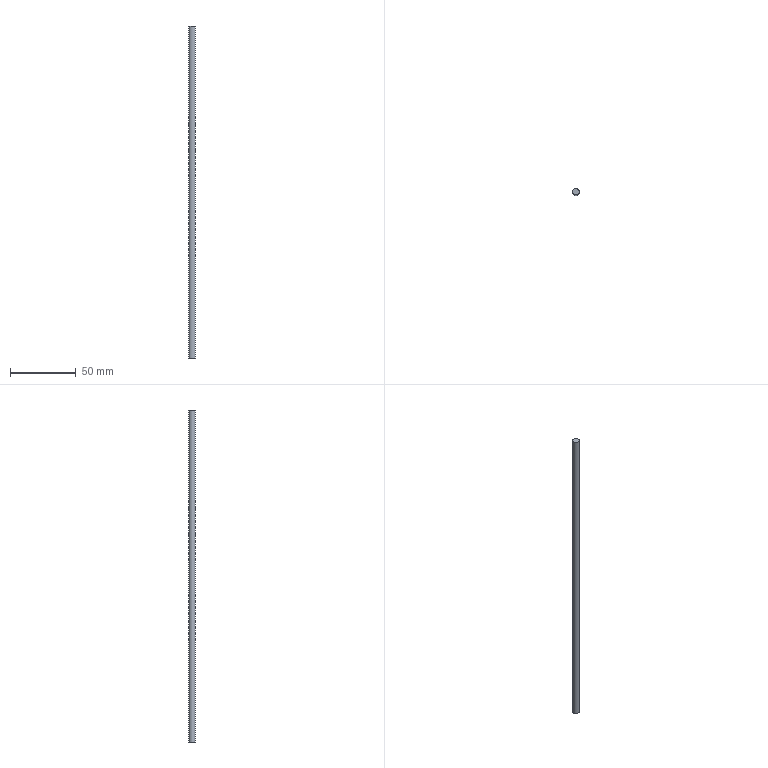Part | STEP file | gslz 2016.10.28-13_id302_x_t | 1 solid | 3 faces | box 5 x 5 x 252 mm | volume 4948 mm3 | plane 2 | cylinder 1 | commonest cylinder face diameters 5 x1
STEP:
#1=CARTESIAN_POINT('',(0.,0.,0.));
#2=DIRECTION('',(0.,0.,1.));
#3=DIRECTION('',(1.,0.,0.));
#4=AXIS2_PLACEMENT_3D('',#1,#2,#3);
#5=CARTESIAN_POINT('',(-229.514,212.012,73.));
#6=VERTEX_POINT('',#5);
#7=CARTESIAN_POINT('',(-234.496,212.311,73.));
#8=VERTEX_POINT('',#7);
#9=CARTESIAN_POINT('',(-232.014,212.012,73.));
#10=DIRECTION('',(0.,0.,-1.));
#11=DIRECTION('',(1.,0.,0.));
#12=AXIS2_PLACEMENT_3D('',#9,#10,#11);
#13=CIRCLE('',#12,2.5);
#14=CARTESIAN_POINT('',(-232.014,212.012,21.));
#15=DIRECTION('',(0.,0.,-1.));
#16=DIRECTION('',(0.,1.,0.));
#17=AXIS2_PLACEMENT_3D('',#14,#15,#16);
#18=CYLINDRICAL_SURFACE('',#17,2.5);
#19=CARTESIAN_POINT('',(7.854,-52.));
#20=DIRECTION('',(1.,0.));
#21=VECTOR('',#20,1.);
#22=LINE('',#19,#21);
#23=(GEOMETRIC_REPRESENTATION_CONTEXT(2)PARAMETRIC_REPRESENTATION_CONTEXT()REPRESENTATION_CONTEXT('',''));
#24=DEFINITIONAL_REPRESENTATION('',(#22),#23);
#25=PCURVE('',#18,#24);
#26=CARTESIAN_POINT('',(-1520.,950.,73.));
#27=DIRECTION('',(0.,0.,1.));
#28=DIRECTION('',(1.,0.,0.));
#29=AXIS2_PLACEMENT_3D('',#26,#27,#28);
#30=PLANE('',#29);
#31=CARTESIAN_POINT('',(1290.486,-737.988));
#32=CARTESIAN_POINT('',(1290.486,-742.318));
#33=CARTESIAN_POINT('',(1286.736,-740.153));
#34=CARTESIAN_POINT('',(1282.986,-737.988));
#35=CARTESIAN_POINT('',(1286.736,-735.823));
#36=CARTESIAN_POINT('',(1290.486,-733.658));
#37=CARTESIAN_POINT('',(1290.486,-737.988));
#38=(BOUNDED_CURVE()B_SPLINE_CURVE(2,(#31,#32,#33,#34,#35,#36,#37),.UNSPECIFIED.,.T.,.F.)B_SPLINE_CURVE_WITH_KNOTS((1,2,2,2,2,1),(-2.094,0.,2.094,4.189,6.283,8.378),.UNSPECIFIED.)CURVE()GEOMETRIC_REPRESENTATION_ITEM()RATIONAL_B_SPLINE_CURVE((1.,0.5,1.,0.5,1.,0.5,1.))REPRESENTATION_ITEM(''));
#39=(GEOMETRIC_REPRESENTATION_CONTEXT(2)PARAMETRIC_REPRESENTATION_CONTEXT()REPRESENTATION_CONTEXT('',''));
#40=DEFINITIONAL_REPRESENTATION('',(#38),#39);
#41=PCURVE('',#30,#40);
#42=SURFACE_CURVE('',#13,(#25,#41),.PCURVE_S1.);
#43=EDGE_CURVE('',#6,#8,#42,.T.);
#44=ORIENTED_EDGE('',*,*,#43,.T.);
#45=CARTESIAN_POINT('',(-234.496,212.311,-179.));
#46=VERTEX_POINT('',#45);
#47=CARTESIAN_POINT('',(-234.496,212.311,73.));
#48=CARTESIAN_POINT('',(-234.496,212.311,-179.));
#49=B_SPLINE_CURVE_WITH_KNOTS('',1,(#47,#48),.UNSPECIFIED.,.F.,.F.,(2,2),(-52.,200.),.PIECEWISE_BEZIER_KNOTS.);
#50=CARTESIAN_POINT('',(11.116,0.));
#51=DIRECTION('',(0.,1.));
#52=VECTOR('',#51,1.);
#53=LINE('',#50,#52);
#54=(GEOMETRIC_REPRESENTATION_CONTEXT(2)PARAMETRIC_REPRESENTATION_CONTEXT()REPRESENTATION_CONTEXT('',''));
#55=DEFINITIONAL_REPRESENTATION('',(#53),#54);
#56=PCURVE('',#18,#55);
#57=CARTESIAN_POINT('',(4.833,0.));
#58=DIRECTION('',(0.,1.));
#59=VECTOR('',#58,1.);
#60=LINE('',#57,#59);
#61=(GEOMETRIC_REPRESENTATION_CONTEXT(2)PARAMETRIC_REPRESENTATION_CONTEXT()REPRESENTATION_CONTEXT('',''));
#62=DEFINITIONAL_REPRESENTATION('',(#60),#61);
#63=PCURVE('',#18,#62);
#64=SEAM_CURVE('',#49,(#56,#63),.PCURVE_S1.);
#65=EDGE_CURVE('',#8,#46,#64,.T.);
#66=ORIENTED_EDGE('',*,*,#65,.T.);
#67=CARTESIAN_POINT('',(-232.014,212.012,-179.));
#68=DIRECTION('',(0.,0.,-1.));
#69=DIRECTION('',(-0.9928,0.1199,0.));
#70=AXIS2_PLACEMENT_3D('',#67,#68,#69);
#71=CIRCLE('',#70,2.5);
#72=CARTESIAN_POINT('',(4.833,200.));
#73=DIRECTION('',(1.,0.));
#74=VECTOR('',#73,1.);
#75=LINE('',#72,#74);
#76=(GEOMETRIC_REPRESENTATION_CONTEXT(2)PARAMETRIC_REPRESENTATION_CONTEXT()REPRESENTATION_CONTEXT('',''));
#77=DEFINITIONAL_REPRESENTATION('',(#75),#76);
#78=PCURVE('',#18,#77);
#79=CARTESIAN_POINT('',(-232.014,212.012,-179.));
#80=DIRECTION('',(0.,0.,-1.));
#81=DIRECTION('',(-1.,0.,0.));
#82=AXIS2_PLACEMENT_3D('',#79,#80,#81);
#83=PLANE('',#82);
#84=CARTESIAN_POINT('',(0.,0.));
#85=DIRECTION('',(0.9928,0.1199));
#86=AXIS2_PLACEMENT_2D('',#84,#85);
#87=CIRCLE('',#86,2.5);
#88=(GEOMETRIC_REPRESENTATION_CONTEXT(2)PARAMETRIC_REPRESENTATION_CONTEXT()REPRESENTATION_CONTEXT('',''));
#89=DEFINITIONAL_REPRESENTATION('',(#87),#88);
#90=PCURVE('',#83,#89);
#91=SURFACE_CURVE('',#71,(#78,#90),.PCURVE_S1.);
#92=EDGE_CURVE('',#46,#46,#91,.T.);
#93=ORIENTED_EDGE('',*,*,#92,.F.);
#94=ORIENTED_EDGE('',*,*,#65,.F.);
#95=CARTESIAN_POINT('',(-232.014,212.012,73.));
#96=DIRECTION('',(0.,0.,-1.));
#97=DIRECTION('',(1.,0.,0.));
#98=AXIS2_PLACEMENT_3D('',#95,#96,#97);
#99=CIRCLE('',#98,2.5);
#100=CARTESIAN_POINT('',(1.571,-52.));
#101=DIRECTION('',(1.,0.));
#102=VECTOR('',#101,1.);
#103=LINE('',#100,#102);
#104=(GEOMETRIC_REPRESENTATION_CONTEXT(2)PARAMETRIC_REPRESENTATION_CONTEXT()REPRESENTATION_CONTEXT('',''));
#105=DEFINITIONAL_REPRESENTATION('',(#103),#104);
#106=PCURVE('',#18,#105);
#107=CARTESIAN_POINT('',(1290.486,-737.988));
#108=CARTESIAN_POINT('',(1290.486,-742.318));
#109=CARTESIAN_POINT('',(1286.736,-740.153));
#110=CARTESIAN_POINT('',(1282.986,-737.988));
#111=CARTESIAN_POINT('',(1286.736,-735.823));
#112=CARTESIAN_POINT('',(1290.486,-733.658));
#113=CARTESIAN_POINT('',(1290.486,-737.988));
#114=(BOUNDED_CURVE()B_SPLINE_CURVE(2,(#107,#108,#109,#110,#111,#112,#113),.UNSPECIFIED.,.T.,.F.)B_SPLINE_CURVE_WITH_KNOTS((1,2,2,2,2,1),(-2.094,0.,2.094,4.189,6.283,8.378),.UNSPECIFIED.)CURVE()GEOMETRIC_REPRESENTATION_ITEM()RATIONAL_B_SPLINE_CURVE((1.,0.5,1.,0.5,1.,0.5,1.))REPRESENTATION_ITEM(''));
#115=(GEOMETRIC_REPRESENTATION_CONTEXT(2)PARAMETRIC_REPRESENTATION_CONTEXT()REPRESENTATION_CONTEXT('',''));
#116=DEFINITIONAL_REPRESENTATION('',(#114),#115);
#117=PCURVE('',#30,#116);
#118=SURFACE_CURVE('',#99,(#106,#117),.PCURVE_S1.);
#119=EDGE_CURVE('',#8,#6,#118,.T.);
#120=ORIENTED_EDGE('',*,*,#119,.T.);
#121=EDGE_LOOP('',(#44,#66,#93,#94,#120));
#122=FACE_BOUND('',#121,.T.);
#123=ADVANCED_FACE('',(#122),#18,.T.);
#124=ORIENTED_EDGE('',*,*,#43,.F.);
#125=ORIENTED_EDGE('',*,*,#119,.F.);
#126=EDGE_LOOP('',(#124,#125));
#127=FACE_BOUND('',#126,.T.);
#128=ADVANCED_FACE('',(#127),#30,.T.);
#129=ORIENTED_EDGE('',*,*,#92,.T.);
#130=EDGE_LOOP('',(#129));
#131=FACE_BOUND('',#130,.T.);
#132=ADVANCED_FACE('',(#131),#83,.T.);
#133=CLOSED_SHELL('',(#123,#128,#132));
#134=MANIFOLD_SOLID_BREP('',#133);
#135=(LENGTH_UNIT()NAMED_UNIT(*)SI_UNIT(.MILLI.,.METRE.));
#136=UNCERTAINTY_MEASURE_WITH_UNIT(LENGTH_MEASURE(0.000005),#135,'','');
#137=(NAMED_UNIT(*)PLANE_ANGLE_UNIT()SI_UNIT($,.RADIAN.));
#138=(NAMED_UNIT(*)SI_UNIT($,.STERADIAN.)SOLID_ANGLE_UNIT());
#139=(GEOMETRIC_REPRESENTATION_CONTEXT(3)GLOBAL_UNCERTAINTY_ASSIGNED_CONTEXT((#136))GLOBAL_UNIT_ASSIGNED_CONTEXT((#135,#137,#138))REPRESENTATION_CONTEXT('',''));
#140=ADVANCED_BREP_SHAPE_REPRESENTATION('',(#4,#134),#139);